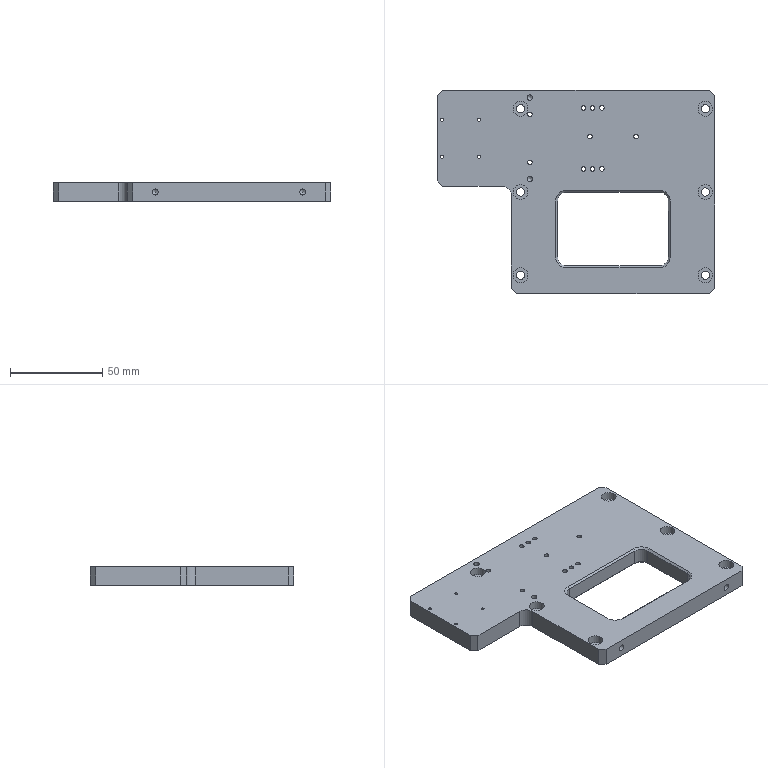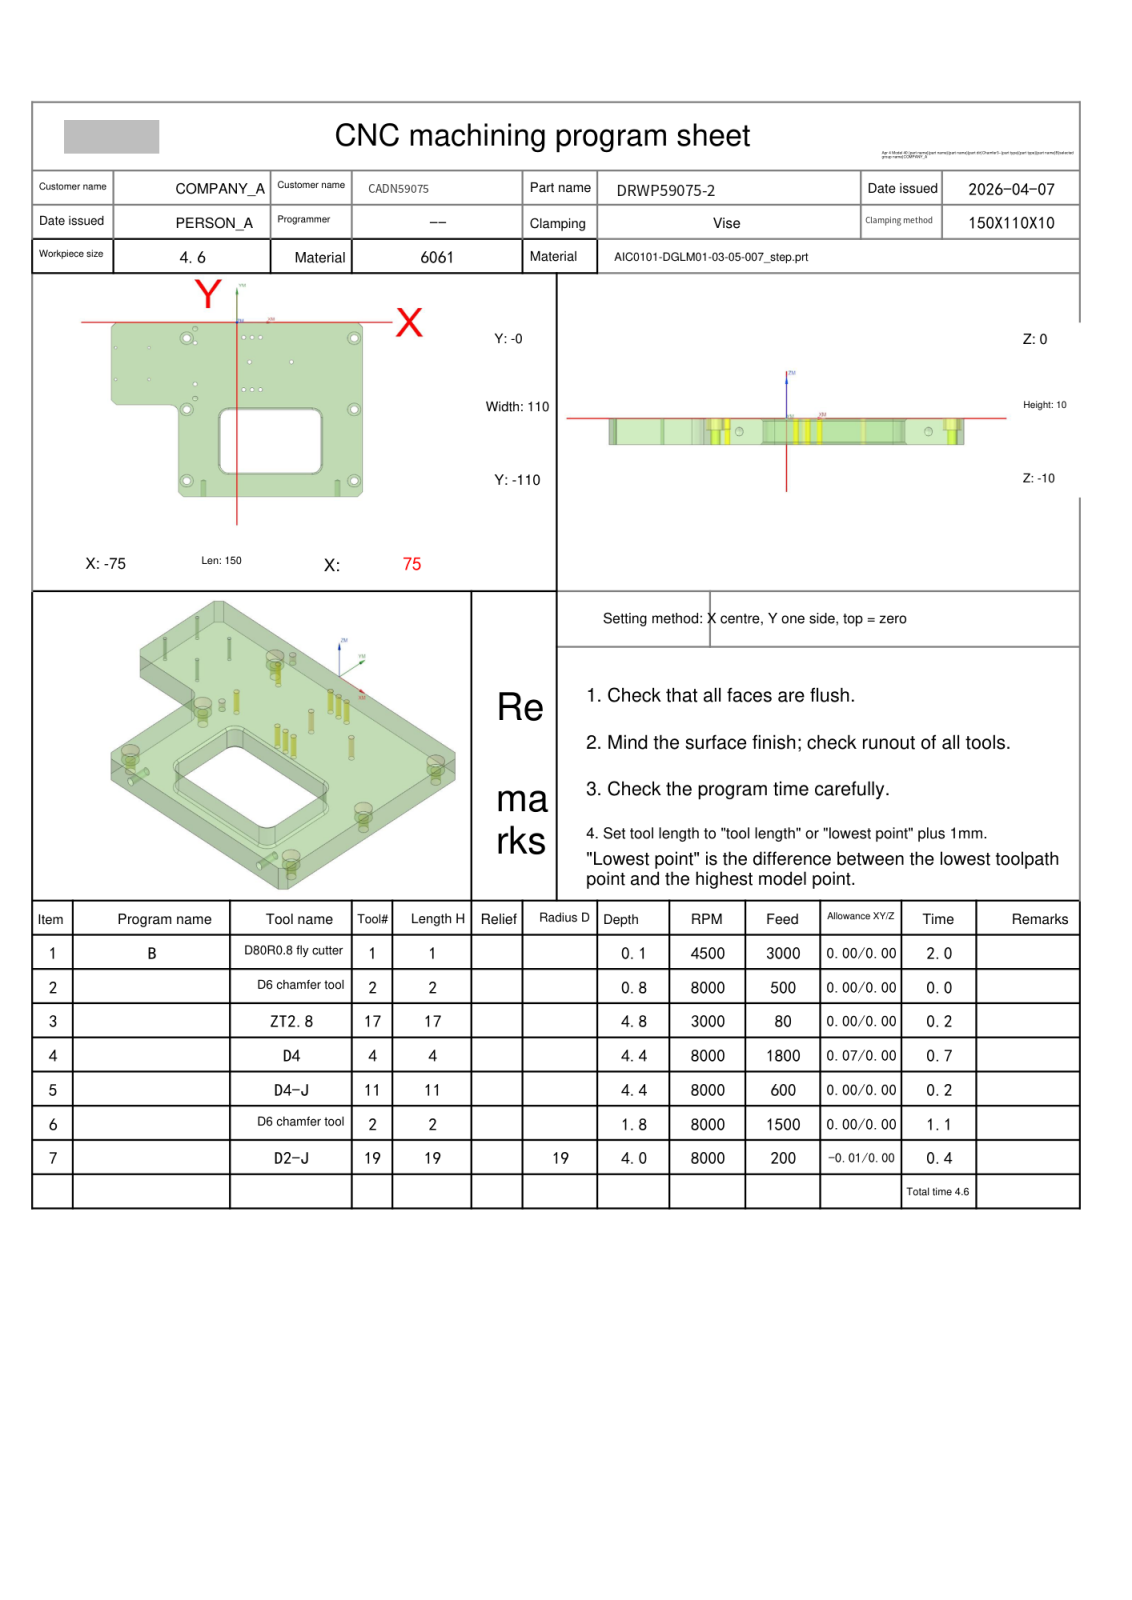NC program | NX | posted by the shop | part box 150 x 110 x 10 mm
Whole program:
%
O0001
(Machine time: 5.89 MIN)
(===Total Tool:6===)
(T1=D80R0.8 fly cutter D=80.  R=0.8  D-  H01 Z=0.    )
(T2=D6 chamfer tool   D=6.   R=0.   D-  H02 Z=-1.8  )
(T17=ZT2.8  D=2.8  DR_a=118 D-  H17 Z=-4.8  )
(T4=D4      D=4.   R=0.   D-  H04 Z=-4.4  )
(T11=D4-J   D=4.   R=0.   D-  H11 Z=-4.4  )
(T19=D2-J   D=2.   R=0.   D19 H19 Z=-4.   )
G80 G90 G17 G49 G40
G91 G28 Z0
M01
N1 T01 M06
(D80R0.8 fly cutter  D=80. R=0.8 H=01 ce=0.20 di=0.10)
G00 G90 G54 X-127. Y-7.5 M03 S4500
G43 H01 Z20.
M08
Z3.525
G01 Z1.525 F3000.
X-115.
X107.8
G02 X115. Y-14.7 I0.0 J-7.2
G01 Y-47.8
G02 X107.8 Y-55. I-7.2 J0.0
G01 X-107.8
G03 X-115. Y-62.2 I0.0 J-7.2
G01 Y-95.3
G03 X-107.8 Y-102.5 I7.2 J0.0
G01 X115.
X127.
Z3.525
G00 Z5.
X-127. Y-7.5
Z3.05
G01 Z1.05
X-115.
X107.8
G02 X115. Y-14.7 I0.0 J-7.2
G01 Y-47.8
G02 X107.8 Y-55. I-7.2 J0.0
G01 X-107.8
G03 X-115. Y-62.2 I0.0 J-7.2
G01 Y-95.3
G03 X-107.8 Y-102.5 I7.2 J0.0
G01 X115.
X127.
Z3.05
G00 Z4.525
X-127. Y-7.5
Z2.575
G01 Z.575
X-115.
X107.8
G02 X115. Y-14.7 I0.0 J-7.2
G01 Y-47.8
G02 X107.8 Y-55. I-7.2 J0.0
G01 X-107.8
G03 X-115. Y-62.2 I0.0 J-7.2
G01 Y-95.3
G03 X-107.8 Y-102.5 I7.2 J0.0
G01 X115.
X127.
Z2.575
G00 Z4.05
X-127. Y-7.5
Z2.1
G01 Z.1
X-115.
X107.8
G02 X115. Y-14.7 I0.0 J-7.2
G01 Y-47.8
G02 X107.8 Y-55. I-7.2 J0.0
G01 X-107.8
G03 X-115. Y-62.2 I0.0 J-7.2
G01 Y-95.3
G03 X-107.8 Y-102.5 I7.2 J0.0
G01 X115.
X127.
Z2.1
G00 Z20.
G00 G90 X-127. Y-7.5 M03 S4500
Z20.
Z2.
G01 Z0.0 F1000.
X-115.
X115.
Y-55.
X-115.
Y-102.5
X115.
X127.
Z2.
G00 Z20.
G91 G28 Z0.0
M05
M09
G91 G28 Z0.0
M01
N2 T02 M06
(D6 chamfer tool  D=6. R=0. H=02 ce=0.00 di=0.00)
G00 G90 G54 X-25. Y-4. M03 S8000
G43 H02 Z20.
M08
G98 G81 X-25. Y-4. Z-.8 R1. F500.
Y-48.
G80
G00 Z20.
G91 G28 Z0.0
M05
M09
G91 G28 Z0.0
M01
N3 T17 M06
(ZT2.8 D=2.8 DR_a=118 H=17)
G00 G90 G54 X-25. Y-4. M03 S3000
G43 H17 Z20.
M08
G98 G83 X-25. Y-4. Z-4.801 R1. F80. Q3.
Y-48.
G80
G00 Z20.
G91 G28 Z0.0
M05
M09
G91 G28 Z0.0
M01
N4 T04 M06
(D4  D=4. R=0. H=04 ce=0.07 di=0.00)
G00 G90 G54 X-30. Y-100. M03 S8000
G43 H04 Z20.
M08
Z.3
G03 X-29.035 Y-100.965 I.965 J0.0 F1800.
X-28.07 Y-100. I0.0 J.965
X-28.07 Y-100. Z-.05 I-1.93 J0.0
X-28.07 Y-100. Z-.4 I-1.93 J0.0
X-28.07 Y-100. Z-.75 I-1.93 J0.0
X-28.07 Y-100. Z-1.1 I-1.93 J0.0
X-28.07 Y-100. Z-1.45 I-1.93 J0.0
X-28.07 Y-100. Z-1.8 I-1.93 J0.0
X-28.07 Y-100. Z-2.15 I-1.93 J0.0
X-28.07 Y-100. Z-2.5 I-1.93 J0.0
X-28.07 Y-100. Z-2.85 I-1.93 J0.0
X-28.07 Y-100. Z-3.2 I-1.93 J0.0
X-28.07 Y-100. Z-3.55 I-1.93 J0.0
X-28.07 Y-100. Z-3.9 I-1.93 J0.0
X-28.07 Y-100. Z-4.25 I-1.93 J0.0
X-31.739 Y-99.163 Z-4.4 I-1.93 J0.0
X-31.93 Y-100. I1.739 J-.837
X-30. Y-101.93 I1.93 J0.0
X-28.07 Y-100. I0.0 J1.93
X-30. Y-98.07 I-1.93 J0.0
X-31.739 Y-99.163 I0.0 J-1.93
X-31.834 Y-99.581 I.869 J-.419
X-30.869 Y-100.546 I.965 J0.0
X-30. Y-100. I0.0 J.965
G00 Z20.
Y-55.
Z.3
G03 X-29.035 Y-55.965 I.965 J0.0
X-28.07 Y-55. I0.0 J.965
X-28.07 Y-55. Z-.05 I-1.93 J0.0
X-28.07 Y-55. Z-.4 I-1.93 J0.0
X-28.07 Y-55. Z-.75 I-1.93 J0.0
X-28.07 Y-55. Z-1.1 I-1.93 J0.0
X-28.07 Y-55. Z-1.45 I-1.93 J0.0
X-28.07 Y-55. Z-1.8 I-1.93 J0.0
X-28.07 Y-55. Z-2.15 I-1.93 J0.0
X-28.07 Y-55. Z-2.5 I-1.93 J0.0
X-28.07 Y-55. Z-2.85 I-1.93 J0.0
X-28.07 Y-55. Z-3.2 I-1.93 J0.0
X-28.07 Y-55. Z-3.55 I-1.93 J0.0
X-28.07 Y-55. Z-3.9 I-1.93 J0.0
X-28.07 Y-55. Z-4.25 I-1.93 J0.0
X-31.739 Y-54.163 Z-4.4 I-1.93 J0.0
X-31.93 Y-55. I1.739 J-.837
X-30. Y-56.93 I1.93 J0.0
X-28.07 Y-55. I0.0 J1.93
X-30. Y-53.07 I-1.93 J0.0
X-31.739 Y-54.163 I0.0 J-1.93
X-31.834 Y-54.581 I.869 J-.419
X-30.869 Y-55.546 I.965 J0.0
X-30. Y-55. I0.0 J.965
G00 Z20.
Y-10.
Z.3
G03 X-29.035 Y-10.965 I.965 J0.0
X-28.07 Y-10. I0.0 J.965
X-28.07 Y-10. Z-.05 I-1.93 J0.0
X-28.07 Y-10. Z-.4 I-1.93 J0.0
X-28.07 Y-10. Z-.75 I-1.93 J0.0
X-28.07 Y-10. Z-1.1 I-1.93 J0.0
X-28.07 Y-10. Z-1.45 I-1.93 J0.0
X-28.07 Y-10. Z-1.8 I-1.93 J0.0
X-28.07 Y-10. Z-2.15 I-1.93 J0.0
X-28.07 Y-10. Z-2.5 I-1.93 J0.0
X-28.07 Y-10. Z-2.85 I-1.93 J0.0
X-28.07 Y-10. Z-3.2 I-1.93 J0.0
X-28.07 Y-10. Z-3.55 I-1.93 J0.0
X-28.07 Y-10. Z-3.9 I-1.93 J0.0
X-28.07 Y-10. Z-4.25 I-1.93 J0.0
X-31.739 Y-9.163 Z-4.4 I-1.93 J0.0
X-31.93 Y-10. I1.739 J-.837
X-30. Y-11.93 I1.93 J0.0
X-28.07 Y-10. I0.0 J1.93
X-30. Y-8.07 I-1.93 J0.0
X-31.739 Y-9.163 I0.0 J-1.93
X-31.834 Y-9.581 I.869 J-.419
X-30.869 Y-10.546 I.965 J0.0
X-30. Y-10. I0.0 J.965
G00 Z20.
X70.
Z.3
G03 X70.965 Y-10.965 I.965 J0.0
X71.93 Y-10. I0.0 J.965
X71.93 Y-10. Z-.05 I-1.93 J0.0
X71.93 Y-10. Z-.4 I-1.93 J0.0
X71.93 Y-10. Z-.75 I-1.93 J0.0
X71.93 Y-10. Z-1.1 I-1.93 J0.0
X71.93 Y-10. Z-1.45 I-1.93 J0.0
X71.93 Y-10. Z-1.8 I-1.93 J0.0
X71.93 Y-10. Z-2.15 I-1.93 J0.0
X71.93 Y-10. Z-2.5 I-1.93 J0.0
X71.93 Y-10. Z-2.85 I-1.93 J0.0
X71.93 Y-10. Z-3.2 I-1.93 J0.0
X71.93 Y-10. Z-3.55 I-1.93 J0.0
X71.93 Y-10. Z-3.9 I-1.93 J0.0
X71.93 Y-10. Z-4.25 I-1.93 J0.0
X68.261 Y-9.163 Z-4.4 I-1.93 J0.0
X68.07 Y-10. I1.739 J-.837
X70. Y-11.93 I1.93 J0.0
X71.93 Y-10. I0.0 J1.93
X70. Y-8.07 I-1.93 J0.0
X68.261 Y-9.163 I0.0 J-1.93
X68.166 Y-9.581 I.869 J-.419
X69.131 Y-10.546 I.965 J0.0
X70. Y-10. I0.0 J.965
G00 Z20.
Y-55.
Z.3
G03 X70.965 Y-55.965 I.965 J0.0
X71.93 Y-55. I0.0 J.965
X71.93 Y-55. Z-.05 I-1.93 J0.0
X71.93 Y-55. Z-.4 I-1.93 J0.0
X71.93 Y-55. Z-.75 I-1.93 J0.0
X71.93 Y-55. Z-1.1 I-1.93 J0.0
X71.93 Y-55. Z-1.45 I-1.93 J0.0
X71.93 Y-55. Z-1.8 I-1.93 J0.0
X71.93 Y-55. Z-2.15 I-1.93 J0.0
X71.93 Y-55. Z-2.5 I-1.93 J0.0
X71.93 Y-55. Z-2.85 I-1.93 J0.0
X71.93 Y-55. Z-3.2 I-1.93 J0.0
X71.93 Y-55. Z-3.55 I-1.93 J0.0
X71.93 Y-55. Z-3.9 I-1.93 J0.0
X71.93 Y-55. Z-4.25 I-1.93 J0.0
X68.261 Y-54.163 Z-4.4 I-1.93 J0.0
X68.07 Y-55. I1.739 J-.837
X70. Y-56.93 I1.93 J0.0
X71.93 Y-55. I0.0 J1.93
X70. Y-53.07 I-1.93 J0.0
X68.261 Y-54.163 I0.0 J-1.93
X68.166 Y-54.581 I.869 J-.419
X69.131 Y-55.546 I.965 J0.0
X70. Y-55. I0.0 J.965
G00 Z20.
Y-100.
Z.3
G03 X70.965 Y-100.965 I.965 J0.0
X71.93 Y-100. I0.0 J.965
X71.93 Y-100. Z-.05 I-1.93 J0.0
X71.93 Y-100. Z-.4 I-1.93 J0.0
X71.93 Y-100. Z-.75 I-1.93 J0.0
X71.93 Y-100. Z-1.1 I-1.93 J0.0
X71.93 Y-100. Z-1.45 I-1.93 J0.0
X71.93 Y-100. Z-1.8 I-1.93 J0.0
X71.93 Y-100. Z-2.15 I-1.93 J0.0
X71.93 Y-100. Z-2.5 I-1.93 J0.0
X71.93 Y-100. Z-2.85 I-1.93 J0.0
X71.93 Y-100. Z-3.2 I-1.93 J0.0
X71.93 Y-100. Z-3.55 I-1.93 J0.0
X71.93 Y-100. Z-3.9 I-1.93 J0.0
X71.93 Y-100. Z-4.25 I-1.93 J0.0
X68.261 Y-99.163 Z-4.4 I-1.93 J0.0
X68.07 Y-100. I1.739 J-.837
X70. Y-101.93 I1.93 J0.0
X71.93 Y-100. I0.0 J1.93
X70. Y-98.07 I-1.93 J0.0
X68.261 Y-99.163 I0.0 J-1.93
X68.166 Y-99.581 I.869 J-.419
X69.131 Y-100.546 I.965 J0.0
X70. Y-100. I0.0 J.965
G00 Z20.
G91 G28 Z0.0
M05
M09
G91 G28 Z0.0
M01
N5 T11 M06
(D4-J  D=4. R=0. H=11 ce=0.00 di=0.00)
G00 G90 G54 X-30. Y-100. M03 S8000
G43 H11 Z20.
M08
Z-4.4
G01 X-28.404 Y-100.329 F600.
X-28.336 Y-100.336
G03 X-28. Y-100. I0.0 J.336
X-30. Y-98. I-2. J0.0
X-32. Y-100. I0.0 J-2.
X-30. Y-102. I2. J0.0
X-28. Y-100. I0.0 J2.
X-28.062 Y-99.505 I-2. J0.0
X-28.388 Y-99.252 I-.325 J-.083
G01 X-28.535 Y-99.286
X-30. Y-100.
G00 Z20.
Y-55.
Z-4.4
G01 X-28.404 Y-55.329
X-28.336 Y-55.336
G03 X-28. Y-55. I0.0 J.336
X-30. Y-53. I-2. J0.0
X-32. Y-55. I0.0 J-2.
X-30. Y-57. I2. J0.0
X-28. Y-55. I0.0 J2.
X-28.062 Y-54.505 I-2. J0.0
X-28.388 Y-54.252 I-.325 J-.083
G01 X-28.535 Y-54.286
X-30. Y-55.
G00 Z20.
Y-10.
Z-4.4
G01 X-28.404 Y-10.329
X-28.336 Y-10.336
G03 X-28. Y-10. I0.0 J.336
X-30. Y-8. I-2. J0.0
X-32. Y-10. I0.0 J-2.
X-30. Y-12. I2. J0.0
X-28. Y-10. I0.0 J2.
X-28.062 Y-9.505 I-2. J0.0
X-28.388 Y-9.252 I-.325 J-.083
G01 X-28.535 Y-9.286
X-30. Y-10.
G00 Z20.
X70.
Z-4.4
G01 X71.596 Y-10.329
X71.664 Y-10.336
G03 X72. Y-10. I0.0 J.336
X70. Y-8. I-2. J0.0
X68. Y-10. I0.0 J-2.
X70. Y-12. I2. J0.0
X72. Y-10. I0.0 J2.
X71.938 Y-9.505 I-2. J0.0
X71.612 Y-9.252 I-.325 J-.083
G01 X71.465 Y-9.286
X70. Y-10.
G00 Z20.
Y-55.
Z-4.4
G01 X71.596 Y-55.329
X71.664 Y-55.336
G03 X72. Y-55. I0.0 J.336
X70. Y-53. I-2. J0.0
X68. Y-55. I0.0 J-2.
X70. Y-57. I2. J0.0
X72. Y-55. I0.0 J2.
X71.938 Y-54.505 I-2. J0.0
X71.612 Y-54.252 I-.325 J-.083
G01 X71.465 Y-54.286
X70. Y-55.
G00 Z20.
Y-100.
Z-4.4
G01 X71.596 Y-100.329
X71.664 Y-100.336
G03 X72. Y-100. I0.0 J.336
X70. Y-98. I-2. J0.0
X68. Y-100. I0.0 J-2.
X70. Y-102. I2. J0.0
X72. Y-100. I0.0 J2.
X71.938 Y-99.505 I-2. J0.0
X71.612 Y-99.252 I-.325 J-.083
G01 X71.465 Y-99.286
X70. Y-100.
G00 Z20.
G91 G28 Z0.0
M05
M09
G91 G28 Z0.0
M01
N6 T02 M06
(D6 chamfer tool  D=6. R=0. H=02 ce=0.00 di=0.00)
G00 G90 G54 X-72.5 Y-16. M03 S4500
G43 H02 Z20.
M08
G98 G81 X-72.5 Y-16. Z-1.1 R1. F500.
X-52.5
Y-36.
X-72.5
G80
G00 Z20.
G00 G90 X32.5 Y-25. M03 S8000
Z20.
G98 G81 X32.5 Y-25. Z-1.75 R3. F1000.
X14. Y-9.5
X9.
X4.
X7.5 Y-25.
X14. Y-42.5
X9.
X4.
X-25. Y-39.
Y-13.
G80
G00 Z20.
G00 G90 X-25. Y-4. M03 S8000
Z20.
G98 G81 X-25. Y-4. Z-1.8 R3. F500.
Y-48.
G80
G00 Z20.
G00 G90 X-6.2 Y-92.193 M03 S6500
Z20.
Z-.2
G01 Z-1.7 F1500.
Y-92.5
G03 X-5. Y-93.7 I1.2 J0.0
G01 X45.
G03 X48.7 Y-90. I0.0 J3.7
G01 Y-60.
G03 X45. Y-56.3 I-3.7 J0.0
G01 X-5.
G03 X-6.225 Y-56.509 I0.0 J-3.7
G01 X-6.278 Y-56.528
G03 X-6.58 Y-56.654 I1.278 J-3.472
G01 X-6.701 Y-56.714
G03 X-8.499 Y-58.798 I1.701 J-3.286
G01 X-8.519 Y-58.856
G03 X-8.607 Y-59.178 I3.519 J-1.144
G01 X-8.617 Y-59.22
G03 X-8.7 Y-60. I3.617 J-.78
G01 Y-90.
G03 X-5. Y-93.7 I3.7 J0.0
G01 X-4.6
G03 X-3.4 Y-92.5 I0.0 J1.2
G01 X-6.2 Y-92.7
G03 X-5. Y-93.9 I1.2 J0.0
G01 X45.
G03 X48.9 Y-90. I0.0 J3.9
G01 Y-60.
G03 X45. Y-56.1 I-3.9 J0.0
G01 X-5.
G03 X-6.291 Y-56.32 I0.0 J-3.9
G01 X-6.347 Y-56.34
X-6.387 Y-56.355
G03 X-6.665 Y-56.473 I1.387 J-3.645
G01 X-6.793 Y-56.537
G03 X-8.688 Y-58.733 I1.793 J-3.463
G01 X-8.709 Y-58.794
G03 X-8.802 Y-59.133 I3.709 J-1.206
G01 X-8.812 Y-59.178
G03 X-8.9 Y-60. I3.812 J-.822
G01 Y-90.
G03 X-5. Y-93.9 I3.9 J0.0
G01 X-4.6
G03 X-3.4 Y-92.7 I0.0 J1.2
G01 X-6.2 Y-92.9
G03 X-5. Y-94.1 I1.2 J0.0
G01 X45.
G03 X49.1 Y-90. I0.0 J4.1
G01 Y-60.
G03 X45. Y-55.9 I-4.1 J0.0
G01 X-5.
G03 X-6.357 Y-56.131 I0.0 J-4.1
G01 X-6.416 Y-56.152
X-6.458 Y-56.168
G03 X-6.751 Y-56.293 I1.458 J-3.832
G01 X-6.885 Y-56.359
G03 X-8.878 Y-58.668 I1.885 J-3.641
G01 X-8.899 Y-58.732
G03 X-8.997 Y-59.089 I3.899 J-1.268
G01 X-9.008 Y-59.136
G03 X-9.1 Y-60. I4.008 J-.864
G01 Y-90.
G03 X-5. Y-94.1 I4.1 J0.0
G01 X-4.6
G03 X-3.4 Y-92.9 I0.0 J1.2
G01 X-6.2 Y-93.1
G03 X-5. Y-94.3 I1.2 J0.0
G01 X45.
G03 X49.3 Y-90. I0.0 J4.3
G01 Y-60.
G03 X45. Y-55.7 I-4.3 J0.0
G01 X-5.
G03 X-6.423 Y-55.942 I0.0 J-4.3
G01 X-6.485 Y-55.965
X-6.53 Y-55.981
G03 X-9.067 Y-58.603 I1.53 J-4.019
G01 X-9.089 Y-58.67
G03 X-9.192 Y-59.044 I4.089 J-1.33
G01 X-9.203 Y-59.093
G03 X-9.3 Y-60. I4.203 J-.907
G01 Y-90.
G03 X-5. Y-94.3 I4.3 J0.0
G01 X-4.6
G03 X-3.4 Y-93.1 I0.0 J1.2
G01 Z-.2
G00 Z20.
G00 G90 X-.386 Y1.227 M03 S6500
Z20.
Z.172
G01 Z-1.2 F1500.
G03 X-.1 Y1.027 I1.286 J1.532
G01 X-.054 Y.997
X0.0 Y1.
X72.
X72.259 Y.966
X72.5 Y.866
X72.707 Y.707
X75.707 Y-2.293
X75.866 Y-2.5
X75.966 Y-2.741
X76. Y-3.
Y-107.
X75.966 Y-107.259
X75.866 Y-107.5
X75.707 Y-107.707
X72.707 Y-110.707
X72.5 Y-110.866
X72.259 Y-110.966
X72. Y-111.
X-32.
X-32.259 Y-110.966
X-32.5 Y-110.866
X-32.707 Y-110.707
X-35.707 Y-107.707
X-35.866 Y-107.5
X-35.966 Y-107.259
X-36. Y-107.
Y-57.
G03 X-40. Y-53. I-4. J0.0
G01 X-72.
X-72.259 Y-52.966
X-72.5 Y-52.866
X-72.707 Y-52.707
X-75.707 Y-49.707
X-75.866 Y-49.5
X-75.966 Y-49.259
X-76. Y-49.
Y-3.
X-75.966 Y-2.741
X-75.866 Y-2.5
X-75.707 Y-2.293
X-72.707 Y.707
X-72.5 Y.866
X-72.259 Y.966
X-72. Y1.
X0.0
X.054 Y.997
X.1 Y1.027
G03 X.386 Y1.227 I-1. J1.732
G01 Z.172
G00 Z10.
X-25.344 Y-3.581
Z.447
G01 Z-1.2
G03 X-25.491 Y-3.897 I1.732 J-1.
G01 X-25.512 Y-3.947
X-25.5 Y-4.
G03 X-25. Y-4.5 I.5 J0.0
X-24.5 Y-4. I0.0 J.5
X-25. Y-3.5 I-.5 J0.0
X-25.5 Y-4. I0.0 J-.5
G01 X-25.512 Y-4.053
X-25.491 Y-4.103
G03 X-25.344 Y-4.419 I1.879 J.684
G01 Z.447
G00 Z2.55
X-32.803 Y-9.599
Z.24
G01 Z-1.2
G03 X-32.981 Y-9.898 I1.624 J-1.167
G01 X-33.007 Y-9.946
X-33. Y-10.
G03 X-30. Y-13. I3. J0.0
X-27. Y-10. I0.0 J3.
X-30. Y-7. I-3. J0.0
X-33. Y-10. I0.0 J-3.
G01 X-33.007 Y-10.054
X-32.981 Y-10.102
G03 X-32.803 Y-10.401 I1.802 J.868
G01 Z.24
G00 Z10.
X-25.344 Y-47.581
Z.447
G01 Z-1.2
G03 X-25.491 Y-47.897 I1.732 J-1.
G01 X-25.512 Y-47.947
X-25.5 Y-48.
G03 X-25. Y-48.5 I.5 J0.0
X-24.5 Y-48. I0.0 J.5
X-25. Y-47.5 I-.5 J0.0
X-25.5 Y-48. I0.0 J-.5
G01 X-25.512 Y-48.053
X-25.491 Y-48.103
G03 X-25.344 Y-48.419 I1.879 J.684
G01 Z.447
G00 Z2.55
X-32.803 Y-54.599
Z.24
G01 Z-1.2
G03 X-32.981 Y-54.898 I1.624 J-1.167
G01 X-33.007 Y-54.946
X-33. Y-55.
G03 X-30. Y-58. I3. J0.0
X-27. Y-55. I0.0 J3.
X-30. Y-52. I-3. J0.0
X-33. Y-55. I0.0 J-3.
G01 X-33.007 Y-55.054
X-32.981 Y-55.102
G03 X-32.803 Y-55.401 I1.802 J.868
G01 Z.24
G00 Z10.
Y-99.599
Z.24
G01 Z-1.2
G03 X-32.981 Y-99.898 I1.624 J-1.167
G01 X-33.007 Y-99.946
X-33. Y-100.
G03 X-30. Y-103. I3. J0.0
X-27. Y-100. I0.0 J3.
X-30. Y-97. I-3. J0.0
X-33. Y-100. I0.0 J-3.
G01 X-33.007 Y-100.054
X-32.981 Y-100.102
G03 X-32.803 Y-100.401 I1.802 J.868
G01 Z.24
G00 Z10.
X67.197 Y-99.599
Z.24
G01 Z-1.2
G03 X67.019 Y-99.898 I1.624 J-1.167
G01 X66.993 Y-99.946
X67. Y-100.
G03 X70. Y-103. I3. J0.0
X73. Y-100. I0.0 J3.
X70. Y-97. I-3. J0.0
X67. Y-100. I0.0 J-3.
G01 X66.993 Y-100.054
X67.019 Y-100.102
G03 X67.197 Y-100.401 I1.802 J.868
G01 Z.24
G00 Z10.
Y-54.599
Z.24
G01 Z-1.2
G03 X67.019 Y-54.898 I1.624 J-1.167
G01 X66.993 Y-54.946
X67. Y-55.
G03 X70. Y-58. I3. J0.0
X73. Y-55. I0.0 J3.
X70. Y-52. I-3. J0.0
X67. Y-55. I0.0 J-3.
G01 X66.993 Y-55.054
X67.019 Y-55.102
G03 X67.197 Y-55.401 I1.802 J.868
G01 Z.24
G00 Z10.
Y-9.599
Z.24
G01 Z-1.2
G03 X67.019 Y-9.898 I1.624 J-1.167
G01 X66.993 Y-9.946
X67. Y-10.
G03 X70. Y-13. I3. J0.0
X73. Y-10. I0.0 J3.
X70. Y-7. I-3. J0.0
X67. Y-10. I0.0 J-3.
G01 X66.993 Y-10.054
X67.019 Y-10.102
G03 X67.197 Y-10.401 I1.802 J.868
G01 Z.24
G00 Z20.
G91 G28 Z0.0
M05
M09
G91 G28 Z0.0
M01
N7 T19 M06
(D2-J  D=2. R=0. H=19 ce=-0.01 di=0.00)
G00 G90 G54 X-25. Y-4. M03 S8000
G43 H19 Z20.
M08
Z.5
G41 D19
G01 X-24.864 Y-4.147 F200.
X-24.706 Y-4.216
G03 X-24.49 Y-4. I0.0 J.216
X-24.49 Y-4. Z0.0 I-.51 J0.0
X-24.49 Y-4. Z-.5 I-.51 J0.0
X-24.49 Y-4. Z-1. I-.51 J0.0
X-24.49 Y-4. Z-1.5 I-.51 J0.0
X-24.49 Y-4. Z-2. I-.51 J0.0
X-24.49 Y-4. Z-2.5 I-.51 J0.0
X-24.49 Y-4. Z-3. I-.51 J0.0
X-24.49 Y-4. Z-3.5 I-.51 J0.0
X-24.49 Y-4. Z-4. I-.51 J0.0
X-25. Y-3.49 I-.51 J0.0
X-25.51 Y-4. I0.0 J-.51
X-25. Y-4.51 I.51 J0.0
X-24.49 Y-4. I0.0 J.51
X-24.706 Y-3.784 I-.216 J0.0
G01 X-24.864 Y-3.853
G40 X-25. Y-4.
G00 Z20.
Y-48.
Z.5
G41 D19
G01 X-24.864 Y-48.147
X-24.706 Y-48.216
G03 X-24.49 Y-48. I0.0 J.216
X-24.49 Y-48. Z0.0 I-.51 J0.0
X-24.49 Y-48. Z-.5 I-.51 J0.0
X-24.49 Y-48. Z-1. I-.51 J0.0
X-24.49 Y-48. Z-1.5 I-.51 J0.0
X-24.49 Y-48. Z-2. I-.51 J0.0
X-24.49 Y-48. Z-2.5 I-.51 J0.0
X-24.49 Y-48. Z-3. I-.51 J0.0
X-24.49 Y-48. Z-3.5 I-.51 J0.0
X-24.49 Y-48. Z-4. I-.51 J0.0
X-25. Y-47.49 I-.51 J0.0
X-25.51 Y-48. I0.0 J-.51
X-25. Y-48.51 I.51 J0.0
X-24.49 Y-48. I0.0 J.51
X-24.706 Y-47.784 I-.216 J0.0
G01 X-24.864 Y-47.853
G40 X-25. Y-48.
G00 Z20.
M05
M09
G91 G28 Z0.0
G91 G28 Y0.0
M30
%